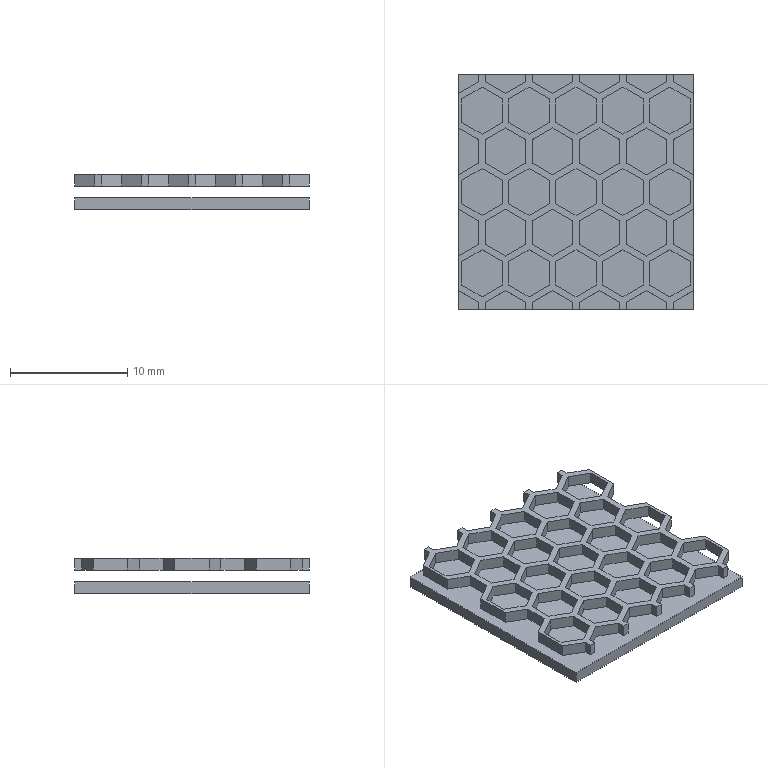Part | SolidWorks | features ICE 6, APattern 1, Extrusion 1 | 2 solids | 214 faces | box 20 x 20 x 3 mm | volume 501.821 mm3 | plane 214